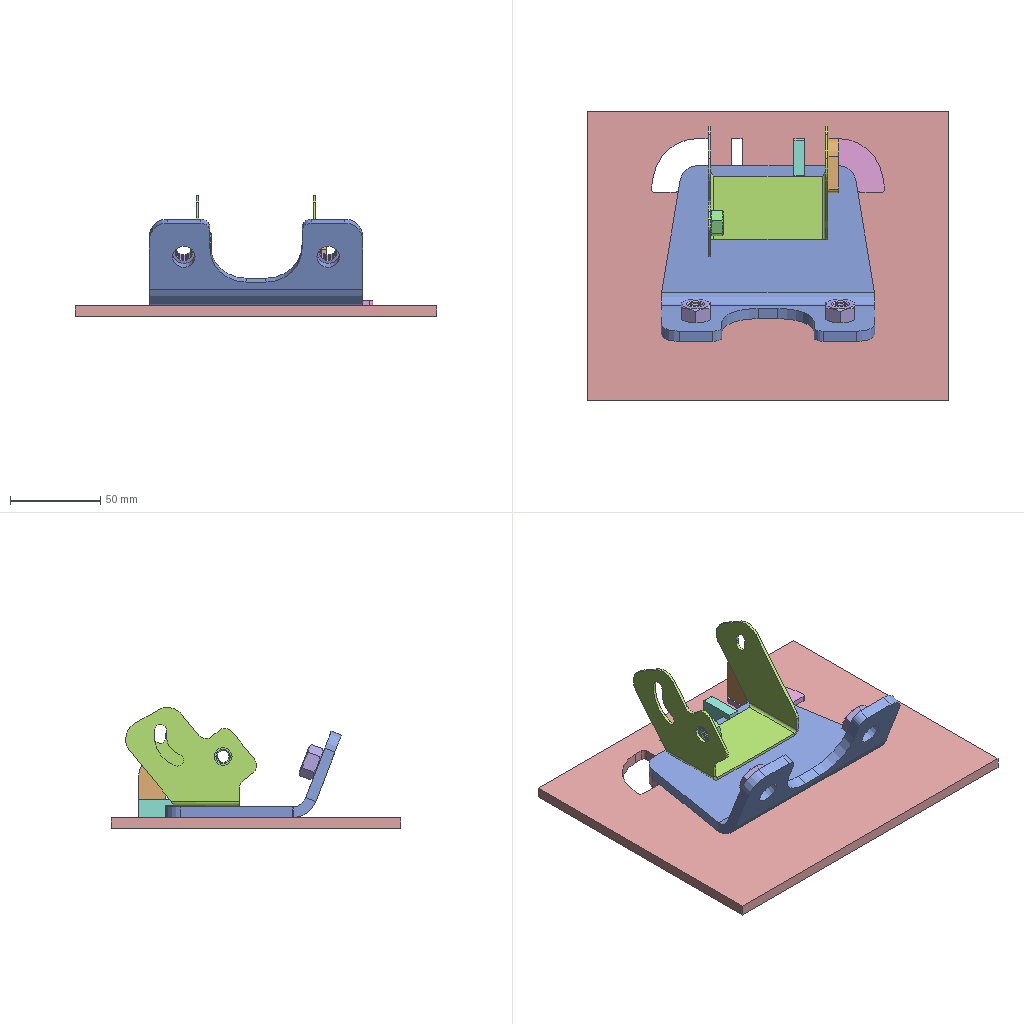Assembly | SolidWorks | 8 different items | 12 placed | box 200 x 160 x 67 mm
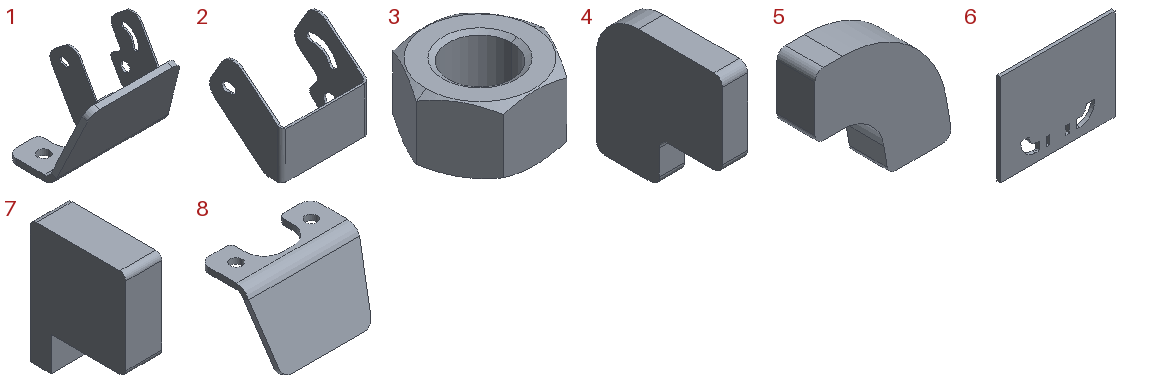Parts list (item | name | quantity | parent item | size | volume | features):
1 | (subassembly) | x1 | - | 118 x 77.569 x 111.373 mm | 80698 mm3 | -
2 | - | x1 | in 1 | 66.4 x 55.014 x 72.708 mm | 10422 mm3 | features ICE 5, Fillet 1, FlatPattern 1, SMBaseFlange 1, SheetMetal 1, UnFold 1
3 | - | x3 | - | 34.641 x 30 x 18 mm | 9644 mm3 | features RevCut 2, Chamfer 1, Extrusion 1, LPattern 1
4 | - | x1 | - | 6 x 30 x 30 mm | 4356 mm3 | features Fillet 1, FlatPattern 1, SMBaseFlange 1, SheetMetal 1
5 | - | x2 | - | 32.296 x 9 x 29.799 mm | 5219 mm3 | features Fillet 1, FlatPattern 1, SMBaseFlange 1, SheetMetal 1
6 | - | x1 | - | 200 x 6 x 160 mm | 183961 mm3 | features Cut 1, FlatPattern 1, ICE 1, SMBaseFlange 1, SheetMetal 1
7 | - | x2 | - | 6 x 16 x 20.7 mm | 1556 mm3 | features Fillet 1, FlatPattern 1, SMBaseFlange 1, SheetMetal 1
8 | - | x1 | in 1 | 118 x 77.569 x 76.575 mm | 70276 mm3 | features FlatPattern 1, SM3dBend 1, SMBaseFlange 1, SheetMetal 1, UnFold 1
Mates (type | each side: item.copy, entity, surface, feature):
In the top assembly
Coincident | 6.1 face plane Base-Flange1 | 8.1 face plane Base-Flange1
Coincident | 6.1 plane | 8.1 edge
Parallel | 6.1 face plane Base-Flange1 | 8.1 face plane Base-Flange1
Coincident | 6.1 face plane Base-Flange1 | 5.1 face plane Base-Flange1
Concentric | 8.1 face cylinder Base-Flange1 | 5.1 face cylinder Base-Flange1
Coincident | 8.1 face plane Base-Flange1 | 5.1 edge
Coincident | 6.1 face plane Cut-Extrude2 | 7.1 face plane Base-Flange1 | 2 times
Coincident | 6.1 face plane Base-Flange1 | 7.1 face plane Base-Flange1
Coincident | 2.1 face plane Base-Flange1 | 4.1 face plane Base-Flange1
Coincident | 5.1 face plane Base-Flange1 | 4.1 face plane Base-Flange1 | 2 times
Coincident | 8.1 face plane Base-Flange1 | 3.1 face plane BaseNut
Concentric | 8.1 edge | 3.1 edge
Parallel | 8.1 face plane Base-Flange1 | 3.1 face plane BaseNut
Coincident | 8.1 face plane Base-Flange1 | 3.2 face plane BaseNut
Concentric | 8.1 edge | 3.2 edge
Parallel | 8.1 face plane Base-Flange1 | 3.2 face plane BaseNut
Coincident | 2.1 face plane Base-Flange1 | 3.3 face plane BaseNut
Concentric | 2.1 edge | 3.3 edge
Perpendicular | 8.1 face plane Base-Flange1 | 3.3 face plane BaseNut
In subassembly 1
Coincident | 8.2 face plane Base-Flange1 | 2.2 face plane Base-Flange1
DistanceDim | 2.2 face plane Base-Flange1 | 8.2 face plane Base-Flange1
DistanceDim | 8.2 face plane Base-Flange1 | 2.2 face cylinder Cut-Extrude3